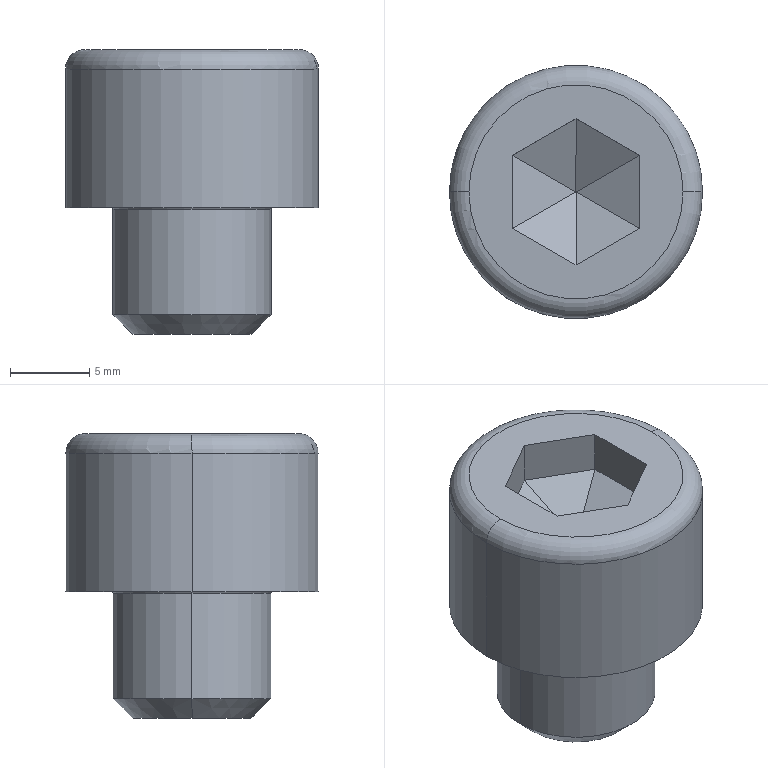Part | STEP file | Socket head cap screw M10x8 | 1 solid | 26 faces | box 16 x 16 x 18 mm | volume 2409 mm3 | plane 16 | torus 4 | cylinder 4 | cone 2 | commonest cylinder face diameters 10 x2 16 x2
STEP:
#1=CARTESIAN_POINT('',(-5.1,0.,0.));
#2=VERTEX_POINT('',#1);
#3=CARTESIAN_POINT('',(5.1,0.,0.));
#4=VERTEX_POINT('',#3);
#5=CARTESIAN_POINT('',(0.,0.,0.));
#6=DIRECTION('',(0.,0.,1.));
#7=DIRECTION('',(1.,0.,0.));
#8=AXIS2_PLACEMENT_3D('',#5,#6,#7);
#9=CIRCLE('',#8,5.1);
#10=EDGE_CURVE('',#2,#4,#9,.T.);
#11=ORIENTED_EDGE('',*,*,#10,.F.);
#12=CARTESIAN_POINT('',(-5.,0.,-0.1));
#13=VERTEX_POINT('',#12);
#14=CARTESIAN_POINT('',(-5.1,0.,-0.1));
#15=DIRECTION('',(0.,1.,0.));
#16=DIRECTION('',(-1.,0.,0.));
#17=AXIS2_PLACEMENT_3D('',#14,#15,#16);
#18=CIRCLE('',#17,0.1);
#19=EDGE_CURVE('',#2,#13,#18,.T.);
#20=ORIENTED_EDGE('',*,*,#19,.T.);
#21=CARTESIAN_POINT('',(5.,0.,-0.1));
#22=VERTEX_POINT('',#21);
#23=CARTESIAN_POINT('',(0.,0.,-0.1));
#24=DIRECTION('',(0.,0.,-1.));
#25=DIRECTION('',(1.,0.,0.));
#26=AXIS2_PLACEMENT_3D('',#23,#24,#25);
#27=CIRCLE('',#26,5.);
#28=EDGE_CURVE('',#22,#13,#27,.T.);
#29=ORIENTED_EDGE('',*,*,#28,.F.);
#30=CARTESIAN_POINT('',(5.1,0.,-0.1));
#31=DIRECTION('',(0.,-1.,0.));
#32=DIRECTION('',(0.,0.,-1.));
#33=AXIS2_PLACEMENT_3D('',#30,#31,#32);
#34=CIRCLE('',#33,0.1);
#35=EDGE_CURVE('',#4,#22,#34,.T.);
#36=ORIENTED_EDGE('',*,*,#35,.F.);
#37=EDGE_LOOP('',(#11,#20,#29,#36));
#38=FACE_OUTER_BOUND('',#37,.T.);
#39=CARTESIAN_POINT('',(0.,0.,-0.1));
#40=DIRECTION('',(0.,0.,1.));
#41=DIRECTION('',(1.,0.,0.));
#42=AXIS2_PLACEMENT_3D('',#39,#40,#41);
#43=TOROIDAL_SURFACE('',#42,5.1,0.1);
#44=ADVANCED_FACE('',(#38),#43,.F.);
#45=CARTESIAN_POINT('',(-8.,0.,8.769));
#46=VERTEX_POINT('',#45);
#47=CARTESIAN_POINT('',(8.,0.,8.769));
#48=VERTEX_POINT('',#47);
#49=CARTESIAN_POINT('',(0.,0.,8.769));
#50=DIRECTION('',(0.,0.,-1.));
#51=DIRECTION('',(1.,0.,0.));
#52=AXIS2_PLACEMENT_3D('',#49,#50,#51);
#53=CIRCLE('',#52,8.);
#54=EDGE_CURVE('',#46,#48,#53,.T.);
#55=ORIENTED_EDGE('',*,*,#54,.F.);
#56=CARTESIAN_POINT('',(-6.769,0.,10.));
#57=VERTEX_POINT('',#56);
#58=CARTESIAN_POINT('',(-6.769,0.,8.769));
#59=DIRECTION('',(0.,1.,0.));
#60=DIRECTION('',(-1.,0.,0.));
#61=AXIS2_PLACEMENT_3D('',#58,#59,#60);
#62=CIRCLE('',#61,1.231);
#63=EDGE_CURVE('',#46,#57,#62,.T.);
#64=ORIENTED_EDGE('',*,*,#63,.T.);
#65=CARTESIAN_POINT('',(6.769,0.,10.));
#66=VERTEX_POINT('',#65);
#67=CARTESIAN_POINT('',(0.,0.,10.));
#68=DIRECTION('',(0.,0.,1.));
#69=DIRECTION('',(1.,0.,0.));
#70=AXIS2_PLACEMENT_3D('',#67,#68,#69);
#71=CIRCLE('',#70,6.769);
#72=EDGE_CURVE('',#66,#57,#71,.T.);
#73=ORIENTED_EDGE('',*,*,#72,.F.);
#74=CARTESIAN_POINT('',(6.769,0.,8.769));
#75=DIRECTION('',(0.,-1.,0.));
#76=DIRECTION('',(0.,0.,-1.));
#77=AXIS2_PLACEMENT_3D('',#74,#75,#76);
#78=CIRCLE('',#77,1.231);
#79=EDGE_CURVE('',#48,#66,#78,.T.);
#80=ORIENTED_EDGE('',*,*,#79,.F.);
#81=EDGE_LOOP('',(#55,#64,#73,#80));
#82=FACE_OUTER_BOUND('',#81,.T.);
#83=CARTESIAN_POINT('',(0.,0.,8.769));
#84=DIRECTION('',(0.,0.,1.));
#85=DIRECTION('',(1.,0.,0.));
#86=AXIS2_PLACEMENT_3D('',#83,#84,#85);
#87=TOROIDAL_SURFACE('',#86,6.769,1.231);
#88=ADVANCED_FACE('',(#82),#87,.T.);
#89=CARTESIAN_POINT('',(-3.75,0.,-8.));
#90=VERTEX_POINT('',#89);
#91=CARTESIAN_POINT('',(3.75,0.,-8.));
#92=VERTEX_POINT('',#91);
#93=CARTESIAN_POINT('',(0.,0.,-8.));
#94=DIRECTION('',(0.,0.,-1.));
#95=DIRECTION('',(-1.,0.,0.));
#96=AXIS2_PLACEMENT_3D('',#93,#94,#95);
#97=CIRCLE('',#96,3.75);
#98=EDGE_CURVE('',#90,#92,#97,.T.);
#99=ORIENTED_EDGE('',*,*,#98,.F.);
#100=CARTESIAN_POINT('',(-5.,0.,-6.75));
#101=VERTEX_POINT('',#100);
#102=CARTESIAN_POINT('',(-3.75,0.,-8.));
#103=DIRECTION('',(-0.7071,0.,0.7071));
#104=VECTOR('',#103,1000.);
#105=LINE('',#102,#104);
#106=EDGE_CURVE('',#90,#101,#105,.T.);
#107=ORIENTED_EDGE('',*,*,#106,.T.);
#108=CARTESIAN_POINT('',(5.,0.,-6.75));
#109=VERTEX_POINT('',#108);
#110=CARTESIAN_POINT('',(0.,0.,-6.75));
#111=DIRECTION('',(0.,0.,1.));
#112=DIRECTION('',(-1.,0.,0.));
#113=AXIS2_PLACEMENT_3D('',#110,#111,#112);
#114=CIRCLE('',#113,5.);
#115=EDGE_CURVE('',#109,#101,#114,.T.);
#116=ORIENTED_EDGE('',*,*,#115,.F.);
#117=CARTESIAN_POINT('',(3.75,0.,-8.));
#118=DIRECTION('',(0.7071,0.,0.7071));
#119=VECTOR('',#118,1000.);
#120=LINE('',#117,#119);
#121=EDGE_CURVE('',#92,#109,#120,.T.);
#122=ORIENTED_EDGE('',*,*,#121,.F.);
#123=EDGE_LOOP('',(#99,#107,#116,#122));
#124=FACE_OUTER_BOUND('',#123,.T.);
#125=CARTESIAN_POINT('',(0.,0.,-8.));
#126=DIRECTION('',(0.,0.,1.));
#127=DIRECTION('',(1.,0.,0.));
#128=AXIS2_PLACEMENT_3D('',#125,#126,#127);
#129=CONICAL_SURFACE('',#128,3.75,0.7854);
#130=ADVANCED_FACE('',(#124),#129,.T.);
#131=ORIENTED_EDGE('',*,*,#115,.T.);
#132=CARTESIAN_POINT('',(-5.,0.,-8.));
#133=DIRECTION('',(0.,0.,1.));
#134=VECTOR('',#133,1000.);
#135=LINE('',#132,#134);
#136=EDGE_CURVE('',#101,#13,#135,.T.);
#137=ORIENTED_EDGE('',*,*,#136,.T.);
#138=CARTESIAN_POINT('',(0.,0.,-0.1));
#139=DIRECTION('',(0.,0.,-1.));
#140=DIRECTION('',(1.,0.,0.));
#141=AXIS2_PLACEMENT_3D('',#138,#139,#140);
#142=CIRCLE('',#141,5.);
#143=EDGE_CURVE('',#13,#22,#142,.T.);
#144=ORIENTED_EDGE('',*,*,#143,.T.);
#145=CARTESIAN_POINT('',(5.,0.,-8.));
#146=DIRECTION('',(0.,0.,1.));
#147=VECTOR('',#146,1000.);
#148=LINE('',#145,#147);
#149=EDGE_CURVE('',#109,#22,#148,.T.);
#150=ORIENTED_EDGE('',*,*,#149,.F.);
#151=EDGE_LOOP('',(#131,#137,#144,#150));
#152=FACE_OUTER_BOUND('',#151,.T.);
#153=CARTESIAN_POINT('',(0.,0.,-8.));
#154=DIRECTION('',(0.,0.,1.));
#155=DIRECTION('',(1.,0.,0.));
#156=AXIS2_PLACEMENT_3D('',#153,#154,#155);
#157=CYLINDRICAL_SURFACE('',#156,5.);
#158=ADVANCED_FACE('',(#152),#157,.T.);
#159=ORIENTED_EDGE('',*,*,#54,.T.);
#160=CARTESIAN_POINT('',(8.,0.,0.));
#161=VERTEX_POINT('',#160);
#162=CARTESIAN_POINT('',(8.,0.,10.));
#163=DIRECTION('',(0.,0.,-1.));
#164=VECTOR('',#163,1000.);
#165=LINE('',#162,#164);
#166=EDGE_CURVE('',#48,#161,#165,.T.);
#167=ORIENTED_EDGE('',*,*,#166,.T.);
#168=CARTESIAN_POINT('',(-8.,0.,0.));
#169=VERTEX_POINT('',#168);
#170=CARTESIAN_POINT('',(0.,0.,0.));
#171=DIRECTION('',(0.,0.,1.));
#172=DIRECTION('',(1.,0.,0.));
#173=AXIS2_PLACEMENT_3D('',#170,#171,#172);
#174=CIRCLE('',#173,8.);
#175=EDGE_CURVE('',#161,#169,#174,.T.);
#176=ORIENTED_EDGE('',*,*,#175,.T.);
#177=CARTESIAN_POINT('',(-8.,0.,10.));
#178=DIRECTION('',(0.,0.,-1.));
#179=VECTOR('',#178,1000.);
#180=LINE('',#177,#179);
#181=EDGE_CURVE('',#46,#169,#180,.T.);
#182=ORIENTED_EDGE('',*,*,#181,.F.);
#183=EDGE_LOOP('',(#159,#167,#176,#182));
#184=FACE_OUTER_BOUND('',#183,.T.);
#185=CARTESIAN_POINT('',(0.,0.,10.));
#186=DIRECTION('',(0.,0.,-1.));
#187=DIRECTION('',(-1.,0.,0.));
#188=AXIS2_PLACEMENT_3D('',#185,#186,#187);
#189=CYLINDRICAL_SURFACE('',#188,8.);
#190=ADVANCED_FACE('',(#184),#189,.T.);
#191=CARTESIAN_POINT('',(0.,0.,0.));
#192=DIRECTION('',(0.,0.,1.));
#193=DIRECTION('',(1.,0.,0.));
#194=AXIS2_PLACEMENT_3D('',#191,#192,#193);
#195=CIRCLE('',#194,5.1);
#196=EDGE_CURVE('',#4,#2,#195,.T.);
#197=ORIENTED_EDGE('',*,*,#196,.T.);
#198=ORIENTED_EDGE('',*,*,#10,.T.);
#199=EDGE_LOOP('',(#197,#198));
#200=FACE_BOUND('',#199,.T.);
#201=CARTESIAN_POINT('',(0.,0.,0.));
#202=DIRECTION('',(0.,0.,1.));
#203=DIRECTION('',(1.,0.,0.));
#204=AXIS2_PLACEMENT_3D('',#201,#202,#203);
#205=CIRCLE('',#204,8.);
#206=EDGE_CURVE('',#169,#161,#205,.T.);
#207=ORIENTED_EDGE('',*,*,#206,.F.);
#208=ORIENTED_EDGE('',*,*,#175,.F.);
#209=EDGE_LOOP('',(#207,#208));
#210=FACE_OUTER_BOUND('',#209,.T.);
#211=CARTESIAN_POINT('',(0.,0.,0.));
#212=DIRECTION('',(0.,0.,1.));
#213=DIRECTION('',(1.,0.,0.));
#214=AXIS2_PLACEMENT_3D('',#211,#212,#213);
#215=PLANE('',#214);
#216=ADVANCED_FACE('',(#200,#210),#215,.F.);
#217=ORIENTED_EDGE('',*,*,#166,.F.);
#218=CARTESIAN_POINT('',(0.,0.,8.769));
#219=DIRECTION('',(0.,0.,-1.));
#220=DIRECTION('',(1.,0.,0.));
#221=AXIS2_PLACEMENT_3D('',#218,#219,#220);
#222=CIRCLE('',#221,8.);
#223=EDGE_CURVE('',#48,#46,#222,.T.);
#224=ORIENTED_EDGE('',*,*,#223,.T.);
#225=ORIENTED_EDGE('',*,*,#181,.T.);
#226=ORIENTED_EDGE('',*,*,#206,.T.);
#227=EDGE_LOOP('',(#217,#224,#225,#226));
#228=FACE_OUTER_BOUND('',#227,.T.);
#229=CARTESIAN_POINT('',(0.,0.,10.));
#230=DIRECTION('',(0.,0.,-1.));
#231=DIRECTION('',(-1.,0.,0.));
#232=AXIS2_PLACEMENT_3D('',#229,#230,#231);
#233=CYLINDRICAL_SURFACE('',#232,8.);
#234=ADVANCED_FACE('',(#228),#233,.T.);
#235=ORIENTED_EDGE('',*,*,#72,.T.);
#236=CARTESIAN_POINT('',(0.,0.,10.));
#237=DIRECTION('',(0.,0.,1.));
#238=DIRECTION('',(1.,0.,0.));
#239=AXIS2_PLACEMENT_3D('',#236,#237,#238);
#240=CIRCLE('',#239,6.769);
#241=EDGE_CURVE('',#57,#66,#240,.T.);
#242=ORIENTED_EDGE('',*,*,#241,.T.);
#243=EDGE_LOOP('',(#235,#242));
#244=FACE_OUTER_BOUND('',#243,.T.);
#245=CARTESIAN_POINT('',(4.,-2.309,10.));
#246=VERTEX_POINT('',#245);
#247=CARTESIAN_POINT('',(4.,2.309,10.));
#248=VERTEX_POINT('',#247);
#249=CARTESIAN_POINT('',(4.,-2.309,10.));
#250=DIRECTION('',(0.,1.,0.));
#251=VECTOR('',#250,1000.);
#252=LINE('',#249,#251);
#253=EDGE_CURVE('',#246,#248,#252,.T.);
#254=ORIENTED_EDGE('',*,*,#253,.F.);
#255=CARTESIAN_POINT('',(0.,-4.619,10.));
#256=VERTEX_POINT('',#255);
#257=CARTESIAN_POINT('',(0.,-4.619,10.));
#258=DIRECTION('',(0.866,0.5,0.));
#259=VECTOR('',#258,1000.);
#260=LINE('',#257,#259);
#261=EDGE_CURVE('',#256,#246,#260,.T.);
#262=ORIENTED_EDGE('',*,*,#261,.F.);
#263=CARTESIAN_POINT('',(-4.,-2.309,10.));
#264=VERTEX_POINT('',#263);
#265=CARTESIAN_POINT('',(-4.,-2.309,10.));
#266=DIRECTION('',(0.866,-0.5,0.));
#267=VECTOR('',#266,1000.);
#268=LINE('',#265,#267);
#269=EDGE_CURVE('',#264,#256,#268,.T.);
#270=ORIENTED_EDGE('',*,*,#269,.F.);
#271=CARTESIAN_POINT('',(-4.,2.309,10.));
#272=VERTEX_POINT('',#271);
#273=CARTESIAN_POINT('',(-4.,2.309,10.));
#274=DIRECTION('',(0.,-1.,0.));
#275=VECTOR('',#274,1000.);
#276=LINE('',#273,#275);
#277=EDGE_CURVE('',#272,#264,#276,.T.);
#278=ORIENTED_EDGE('',*,*,#277,.F.);
#279=CARTESIAN_POINT('',(0.,4.619,10.));
#280=VERTEX_POINT('',#279);
#281=CARTESIAN_POINT('',(0.,4.619,10.));
#282=DIRECTION('',(-0.866,-0.5,0.));
#283=VECTOR('',#282,1000.);
#284=LINE('',#281,#283);
#285=EDGE_CURVE('',#280,#272,#284,.T.);
#286=ORIENTED_EDGE('',*,*,#285,.F.);
#287=CARTESIAN_POINT('',(4.,2.309,10.));
#288=DIRECTION('',(-0.866,0.5,0.));
#289=VECTOR('',#288,1000.);
#290=LINE('',#287,#289);
#291=EDGE_CURVE('',#248,#280,#290,.T.);
#292=ORIENTED_EDGE('',*,*,#291,.F.);
#293=EDGE_LOOP('',(#254,#262,#270,#278,#286,#292));
#294=FACE_BOUND('',#293,.T.);
#295=CARTESIAN_POINT('',(0.,0.,10.));
#296=DIRECTION('',(0.,0.,1.));
#297=DIRECTION('',(1.,0.,0.));
#298=AXIS2_PLACEMENT_3D('',#295,#296,#297);
#299=PLANE('',#298);
#300=ADVANCED_FACE('',(#244,#294),#299,.T.);
#301=CARTESIAN_POINT('',(4.,2.309,7.305));
#302=VERTEX_POINT('',#301);
#303=CARTESIAN_POINT('',(4.,2.309,5.));
#304=DIRECTION('',(0.,0.,1.));
#305=VECTOR('',#304,1000.);
#306=LINE('',#303,#305);
#307=EDGE_CURVE('',#302,#248,#306,.T.);
#308=ORIENTED_EDGE('',*,*,#307,.F.);
#309=CARTESIAN_POINT('',(4.,-2.309,7.305));
#310=VERTEX_POINT('',#309);
#311=CARTESIAN_POINT('',(4.,-2.309,7.305));
#312=DIRECTION('',(0.,-1.,0.));
#313=VECTOR('',#312,1000.);
#314=LINE('',#311,#313);
#315=EDGE_CURVE('',#302,#310,#314,.T.);
#316=ORIENTED_EDGE('',*,*,#315,.T.);
#317=CARTESIAN_POINT('',(4.,-2.309,5.));
#318=DIRECTION('',(0.,0.,1.));
#319=VECTOR('',#318,1000.);
#320=LINE('',#317,#319);
#321=EDGE_CURVE('',#310,#246,#320,.T.);
#322=ORIENTED_EDGE('',*,*,#321,.T.);
#323=ORIENTED_EDGE('',*,*,#253,.T.);
#324=EDGE_LOOP('',(#308,#316,#322,#323));
#325=FACE_OUTER_BOUND('',#324,.T.);
#326=CARTESIAN_POINT('',(4.,-2.309,5.));
#327=DIRECTION('',(1.,0.,0.));
#328=DIRECTION('',(0.,1.,0.));
#329=AXIS2_PLACEMENT_3D('',#326,#327,#328);
#330=PLANE('',#329);
#331=ADVANCED_FACE('',(#325),#330,.F.);
#332=ORIENTED_EDGE('',*,*,#321,.F.);
#333=CARTESIAN_POINT('',(0.,-4.619,7.305));
#334=VERTEX_POINT('',#333);
#335=CARTESIAN_POINT('',(0.,-4.619,7.305));
#336=DIRECTION('',(-0.866,-0.5,0.));
#337=VECTOR('',#336,1000.);
#338=LINE('',#335,#337);
#339=EDGE_CURVE('',#310,#334,#338,.T.);
#340=ORIENTED_EDGE('',*,*,#339,.T.);
#341=CARTESIAN_POINT('',(0.,-4.619,5.));
#342=DIRECTION('',(0.,0.,1.));
#343=VECTOR('',#342,1000.);
#344=LINE('',#341,#343);
#345=EDGE_CURVE('',#334,#256,#344,.T.);
#346=ORIENTED_EDGE('',*,*,#345,.T.);
#347=ORIENTED_EDGE('',*,*,#261,.T.);
#348=EDGE_LOOP('',(#332,#340,#346,#347));
#349=FACE_OUTER_BOUND('',#348,.T.);
#350=CARTESIAN_POINT('',(0.,-4.619,5.));
#351=DIRECTION('',(0.5,-0.866,0.));
#352=DIRECTION('',(0.866,0.5,0.));
#353=AXIS2_PLACEMENT_3D('',#350,#351,#352);
#354=PLANE('',#353);
#355=ADVANCED_FACE('',(#349),#354,.F.);
#356=ORIENTED_EDGE('',*,*,#345,.F.);
#357=CARTESIAN_POINT('',(-4.,-2.309,7.305));
#358=VERTEX_POINT('',#357);
#359=CARTESIAN_POINT('',(-4.,-2.309,7.305));
#360=DIRECTION('',(-0.866,0.5,0.));
#361=VECTOR('',#360,1000.);
#362=LINE('',#359,#361);
#363=EDGE_CURVE('',#334,#358,#362,.T.);
#364=ORIENTED_EDGE('',*,*,#363,.T.);
#365=CARTESIAN_POINT('',(-4.,-2.309,5.));
#366=DIRECTION('',(0.,0.,1.));
#367=VECTOR('',#366,1000.);
#368=LINE('',#365,#367);
#369=EDGE_CURVE('',#358,#264,#368,.T.);
#370=ORIENTED_EDGE('',*,*,#369,.T.);
#371=ORIENTED_EDGE('',*,*,#269,.T.);
#372=EDGE_LOOP('',(#356,#364,#370,#371));
#373=FACE_OUTER_BOUND('',#372,.T.);
#374=CARTESIAN_POINT('',(-4.,-2.309,5.));
#375=DIRECTION('',(-0.5,-0.866,0.));
#376=DIRECTION('',(0.866,-0.5,0.));
#377=AXIS2_PLACEMENT_3D('',#374,#375,#376);
#378=PLANE('',#377);
#379=ADVANCED_FACE('',(#373),#378,.F.);
#380=ORIENTED_EDGE('',*,*,#369,.F.);
#381=CARTESIAN_POINT('',(-4.,2.309,7.305));
#382=VERTEX_POINT('',#381);
#383=CARTESIAN_POINT('',(-4.,2.309,7.305));
#384=DIRECTION('',(0.,1.,0.));
#385=VECTOR('',#384,1000.);
#386=LINE('',#383,#385);
#387=EDGE_CURVE('',#358,#382,#386,.T.);
#388=ORIENTED_EDGE('',*,*,#387,.T.);
#389=CARTESIAN_POINT('',(-4.,2.309,5.));
#390=DIRECTION('',(0.,0.,1.));
#391=VECTOR('',#390,1000.);
#392=LINE('',#389,#391);
#393=EDGE_CURVE('',#382,#272,#392,.T.);
#394=ORIENTED_EDGE('',*,*,#393,.T.);
#395=ORIENTED_EDGE('',*,*,#277,.T.);
#396=EDGE_LOOP('',(#380,#388,#394,#395));
#397=FACE_OUTER_BOUND('',#396,.T.);
#398=CARTESIAN_POINT('',(-4.,2.309,5.));
#399=DIRECTION('',(-1.,0.,0.));
#400=DIRECTION('',(0.,0.,1.));
#401=AXIS2_PLACEMENT_3D('',#398,#399,#400);
#402=PLANE('',#401);
#403=ADVANCED_FACE('',(#397),#402,.F.);
#404=ORIENTED_EDGE('',*,*,#393,.F.);
#405=CARTESIAN_POINT('',(0.,4.619,7.305));
#406=VERTEX_POINT('',#405);
#407=CARTESIAN_POINT('',(0.,4.619,7.305));
#408=DIRECTION('',(0.866,0.5,0.));
#409=VECTOR('',#408,1000.);
#410=LINE('',#407,#409);
#411=EDGE_CURVE('',#382,#406,#410,.T.);
#412=ORIENTED_EDGE('',*,*,#411,.T.);
#413=CARTESIAN_POINT('',(0.,4.619,5.));
#414=DIRECTION('',(0.,0.,1.));
#415=VECTOR('',#414,1000.);
#416=LINE('',#413,#415);
#417=EDGE_CURVE('',#406,#280,#416,.T.);
#418=ORIENTED_EDGE('',*,*,#417,.T.);
#419=ORIENTED_EDGE('',*,*,#285,.T.);
#420=EDGE_LOOP('',(#404,#412,#418,#419));
#421=FACE_OUTER_BOUND('',#420,.T.);
#422=CARTESIAN_POINT('',(0.,4.619,5.));
#423=DIRECTION('',(-0.5,0.866,0.));
#424=DIRECTION('',(-0.866,-0.5,0.));
#425=AXIS2_PLACEMENT_3D('',#422,#423,#424);
#426=PLANE('',#425);
#427=ADVANCED_FACE('',(#421),#426,.F.);
#428=ORIENTED_EDGE('',*,*,#417,.F.);
#429=CARTESIAN_POINT('',(4.,2.309,7.305));
#430=DIRECTION('',(0.866,-0.5,0.));
#431=VECTOR('',#430,1000.);
#432=LINE('',#429,#431);
#433=EDGE_CURVE('',#406,#302,#432,.T.);
#434=ORIENTED_EDGE('',*,*,#433,.T.);
#435=ORIENTED_EDGE('',*,*,#307,.T.);
#436=ORIENTED_EDGE('',*,*,#291,.T.);
#437=EDGE_LOOP('',(#428,#434,#435,#436));
#438=FACE_OUTER_BOUND('',#437,.T.);
#439=CARTESIAN_POINT('',(4.,2.309,5.));
#440=DIRECTION('',(0.5,0.866,0.));
#441=DIRECTION('',(-0.866,0.5,0.));
#442=AXIS2_PLACEMENT_3D('',#439,#440,#441);
#443=PLANE('',#442);
#444=ADVANCED_FACE('',(#438),#443,.F.);
#445=CARTESIAN_POINT('',(0.,0.007851,5.));
#446=VERTEX_POINT('',#445);
#447=CARTESIAN_POINT('',(-0.006799,0.003926,5.));
#448=VERTEX_POINT('',#447);
#449=CARTESIAN_POINT('',(-0.0034,0.005888,5.));
#450=DIRECTION('',(-0.866,-0.5,0.));
#451=VECTOR('',#450,1000.);
#452=LINE('',#449,#451);
#453=EDGE_CURVE('',#446,#448,#452,.T.);
#454=ORIENTED_EDGE('',*,*,#453,.T.);
#455=CARTESIAN_POINT('',(-0.006799,-0.003926,5.));
#456=VERTEX_POINT('',#455);
#457=CARTESIAN_POINT('',(-0.006799,0.,5.));
#458=DIRECTION('',(0.,-1.,0.));
#459=VECTOR('',#458,1000.);
#460=LINE('',#457,#459);
#461=EDGE_CURVE('',#448,#456,#460,.T.);
#462=ORIENTED_EDGE('',*,*,#461,.T.);
#463=CARTESIAN_POINT('',(0.,-0.007851,5.));
#464=VERTEX_POINT('',#463);
#465=CARTESIAN_POINT('',(-0.0034,-0.005888,5.));
#466=DIRECTION('',(0.866,-0.5,0.));
#467=VECTOR('',#466,1000.);
#468=LINE('',#465,#467);
#469=EDGE_CURVE('',#456,#464,#468,.T.);
#470=ORIENTED_EDGE('',*,*,#469,.T.);
#471=CARTESIAN_POINT('',(0.006799,-0.003926,5.));
#472=VERTEX_POINT('',#471);
#473=CARTESIAN_POINT('',(0.0034,-0.005888,5.));
#474=DIRECTION('',(0.866,0.5,0.));
#475=VECTOR('',#474,1000.);
#476=LINE('',#473,#475);
#477=EDGE_CURVE('',#464,#472,#476,.T.);
#478=ORIENTED_EDGE('',*,*,#477,.T.);
#479=CARTESIAN_POINT('',(0.006799,0.003926,5.));
#480=VERTEX_POINT('',#479);
#481=CARTESIAN_POINT('',(0.006799,0.,5.));
#482=DIRECTION('',(0.,1.,0.));
#483=VECTOR('',#482,1000.);
#484=LINE('',#481,#483);
#485=EDGE_CURVE('',#472,#480,#484,.T.);
#486=ORIENTED_EDGE('',*,*,#485,.T.);
#487=CARTESIAN_POINT('',(0.0034,0.005888,5.));
#488=DIRECTION('',(-0.866,0.5,0.));
#489=VECTOR('',#488,1000.);
#490=LINE('',#487,#489);
#491=EDGE_CURVE('',#480,#446,#490,.T.);
#492=ORIENTED_EDGE('',*,*,#491,.T.);
#493=EDGE_LOOP('',(#454,#462,#470,#478,#486,#492));
#494=FACE_OUTER_BOUND('',#493,.T.);
#495=CARTESIAN_POINT('',(0.,0.,5.));
#496=DIRECTION('',(0.,0.,1.));
#497=DIRECTION('',(1.,0.,0.));
#498=AXIS2_PLACEMENT_3D('',#495,#496,#497);
#499=PLANE('',#498);
#500=ADVANCED_FACE('',(#494),#499,.T.);
#501=ORIENTED_EDGE('',*,*,#136,.F.);
#502=CARTESIAN_POINT('',(0.,0.,-6.75));
#503=DIRECTION('',(0.,0.,1.));
#504=DIRECTION('',(-1.,0.,0.));
#505=AXIS2_PLACEMENT_3D('',#502,#503,#504);
#506=CIRCLE('',#505,5.);
#507=EDGE_CURVE('',#101,#109,#506,.T.);
#508=ORIENTED_EDGE('',*,*,#507,.T.);
#509=ORIENTED_EDGE('',*,*,#149,.T.);
#510=ORIENTED_EDGE('',*,*,#28,.T.);
#511=EDGE_LOOP('',(#501,#508,#509,#510));
#512=FACE_OUTER_BOUND('',#511,.T.);
#513=CARTESIAN_POINT('',(0.,0.,-8.));
#514=DIRECTION('',(0.,0.,1.));
#515=DIRECTION('',(1.,0.,0.));
#516=AXIS2_PLACEMENT_3D('',#513,#514,#515);
#517=CYLINDRICAL_SURFACE('',#516,5.);
#518=ADVANCED_FACE('',(#512),#517,.T.);
#519=CARTESIAN_POINT('',(0.,0.,-8.));
#520=DIRECTION('',(0.,0.,-1.));
#521=DIRECTION('',(-1.,0.,0.));
#522=AXIS2_PLACEMENT_3D('',#519,#520,#521);
#523=CIRCLE('',#522,3.75);
#524=EDGE_CURVE('',#92,#90,#523,.T.);
#525=ORIENTED_EDGE('',*,*,#524,.T.);
#526=ORIENTED_EDGE('',*,*,#98,.T.);
#527=EDGE_LOOP('',(#525,#526));
#528=FACE_OUTER_BOUND('',#527,.T.);
#529=CARTESIAN_POINT('',(0.,0.,-8.));
#530=DIRECTION('',(0.,0.,-1.));
#531=DIRECTION('',(-1.,0.,0.));
#532=AXIS2_PLACEMENT_3D('',#529,#530,#531);
#533=PLANE('',#532);
#534=ADVANCED_FACE('',(#528),#533,.T.);
#535=ORIENTED_EDGE('',*,*,#106,.F.);
#536=ORIENTED_EDGE('',*,*,#524,.F.);
#537=ORIENTED_EDGE('',*,*,#121,.T.);
#538=ORIENTED_EDGE('',*,*,#507,.F.);
#539=EDGE_LOOP('',(#535,#536,#537,#538));
#540=FACE_OUTER_BOUND('',#539,.T.);
#541=CARTESIAN_POINT('',(0.,0.,-8.));
#542=DIRECTION('',(0.,0.,1.));
#543=DIRECTION('',(1.,0.,0.));
#544=AXIS2_PLACEMENT_3D('',#541,#542,#543);
#545=CONICAL_SURFACE('',#544,3.75,0.7854);
#546=ADVANCED_FACE('',(#540),#545,.T.);
#547=ORIENTED_EDGE('',*,*,#63,.F.);
#548=ORIENTED_EDGE('',*,*,#223,.F.);
#549=ORIENTED_EDGE('',*,*,#79,.T.);
#550=ORIENTED_EDGE('',*,*,#241,.F.);
#551=EDGE_LOOP('',(#547,#548,#549,#550));
#552=FACE_OUTER_BOUND('',#551,.T.);
#553=CARTESIAN_POINT('',(0.,0.,8.769));
#554=DIRECTION('',(0.,0.,1.));
#555=DIRECTION('',(1.,0.,0.));
#556=AXIS2_PLACEMENT_3D('',#553,#554,#555);
#557=TOROIDAL_SURFACE('',#556,6.769,1.231);
#558=ADVANCED_FACE('',(#552),#557,.T.);
#559=CARTESIAN_POINT('',(0.005439,-0.00314,4.999));
#560=DIRECTION('',(-0.7746,0.4472,-0.4472));
#561=VECTOR('',#560,1000.);
#562=LINE('',#559,#561);
#563=EDGE_CURVE('',#310,#472,#562,.T.);
#564=ORIENTED_EDGE('',*,*,#563,.F.);
#565=ORIENTED_EDGE('',*,*,#315,.F.);
#566=CARTESIAN_POINT('',(0.005439,0.00314,4.999));
#567=DIRECTION('',(0.7746,0.4472,0.4472));
#568=VECTOR('',#567,1000.);
#569=LINE('',#566,#568);
#570=EDGE_CURVE('',#480,#302,#569,.T.);
#571=ORIENTED_EDGE('',*,*,#570,.F.);
#572=ORIENTED_EDGE('',*,*,#485,.F.);
#573=EDGE_LOOP('',(#564,#565,#571,#572));
#574=FACE_OUTER_BOUND('',#573,.T.);
#575=CARTESIAN_POINT('',(0.006799,0.,5.));
#576=DIRECTION('',(0.5,0.,-0.866));
#577=DIRECTION('',(0.,1.,0.));
#578=AXIS2_PLACEMENT_3D('',#575,#576,#577);
#579=PLANE('',#578);
#580=ADVANCED_FACE('',(#574),#579,.F.);
#581=ORIENTED_EDGE('',*,*,#570,.T.);
#582=ORIENTED_EDGE('',*,*,#433,.F.);
#583=CARTESIAN_POINT('',(0.,0.006281,4.999));
#584=DIRECTION('',(0.,0.8944,0.4472));
#585=VECTOR('',#584,1000.);
#586=LINE('',#583,#585);
#587=EDGE_CURVE('',#446,#406,#586,.T.);
#588=ORIENTED_EDGE('',*,*,#587,.F.);
#589=ORIENTED_EDGE('',*,*,#491,.F.);
#590=EDGE_LOOP('',(#581,#582,#588,#589));
#591=FACE_OUTER_BOUND('',#590,.T.);
#592=CARTESIAN_POINT('',(0.0034,0.005888,5.));
#593=DIRECTION('',(0.25,0.433,-0.866));
#594=DIRECTION('',(-0.866,0.5,0.));
#595=AXIS2_PLACEMENT_3D('',#592,#593,#594);
#596=PLANE('',#595);
#597=ADVANCED_FACE('',(#591),#596,.F.);
#598=ORIENTED_EDGE('',*,*,#563,.T.);
#599=ORIENTED_EDGE('',*,*,#477,.F.);
#600=CARTESIAN_POINT('',(0.,-0.006281,4.999));
#601=DIRECTION('',(0.,0.8944,-0.4472));
#602=VECTOR('',#601,1000.);
#603=LINE('',#600,#602);
#604=EDGE_CURVE('',#334,#464,#603,.T.);
#605=ORIENTED_EDGE('',*,*,#604,.F.);
#606=ORIENTED_EDGE('',*,*,#339,.F.);
#607=EDGE_LOOP('',(#598,#599,#605,#606));
#608=FACE_OUTER_BOUND('',#607,.T.);
#609=CARTESIAN_POINT('',(0.0034,-0.005888,5.));
#610=DIRECTION('',(0.25,-0.433,-0.866));
#611=DIRECTION('',(0.866,0.5,0.));
#612=AXIS2_PLACEMENT_3D('',#609,#610,#611);
#613=PLANE('',#612);
#614=ADVANCED_FACE('',(#608),#613,.F.);
#615=ORIENTED_EDGE('',*,*,#587,.T.);
#616=ORIENTED_EDGE('',*,*,#411,.F.);
#617=CARTESIAN_POINT('',(-0.005439,0.00314,4.999));
#618=DIRECTION('',(-0.7746,0.4472,0.4472));
#619=VECTOR('',#618,1000.);
#620=LINE('',#617,#619);
#621=EDGE_CURVE('',#448,#382,#620,.T.);
#622=ORIENTED_EDGE('',*,*,#621,.F.);
#623=ORIENTED_EDGE('',*,*,#453,.F.);
#624=EDGE_LOOP('',(#615,#616,#622,#623));
#625=FACE_OUTER_BOUND('',#624,.T.);
#626=CARTESIAN_POINT('',(-0.0034,0.005888,5.));
#627=DIRECTION('',(-0.25,0.433,-0.866));
#628=DIRECTION('',(-0.866,-0.5,0.));
#629=AXIS2_PLACEMENT_3D('',#626,#627,#628);
#630=PLANE('',#629);
#631=ADVANCED_FACE('',(#625),#630,.F.);
#632=ORIENTED_EDGE('',*,*,#604,.T.);
#633=ORIENTED_EDGE('',*,*,#469,.F.);
#634=CARTESIAN_POINT('',(-0.005439,-0.00314,4.999));
#635=DIRECTION('',(0.7746,0.4472,-0.4472));
#636=VECTOR('',#635,1000.);
#637=LINE('',#634,#636);
#638=EDGE_CURVE('',#358,#456,#637,.T.);
#639=ORIENTED_EDGE('',*,*,#638,.F.);
#640=ORIENTED_EDGE('',*,*,#363,.F.);
#641=EDGE_LOOP('',(#632,#633,#639,#640));
#642=FACE_OUTER_BOUND('',#641,.T.);
#643=CARTESIAN_POINT('',(-0.0034,-0.005888,5.));
#644=DIRECTION('',(-0.25,-0.433,-0.866));
#645=DIRECTION('',(0.866,-0.5,0.));
#646=AXIS2_PLACEMENT_3D('',#643,#644,#645);
#647=PLANE('',#646);
#648=ADVANCED_FACE('',(#642),#647,.F.);
#649=ORIENTED_EDGE('',*,*,#621,.T.);
#650=ORIENTED_EDGE('',*,*,#387,.F.);
#651=ORIENTED_EDGE('',*,*,#638,.T.);
#652=ORIENTED_EDGE('',*,*,#461,.F.);
#653=EDGE_LOOP('',(#649,#650,#651,#652));
#654=FACE_OUTER_BOUND('',#653,.T.);
#655=CARTESIAN_POINT('',(-0.006799,0.,5.));
#656=DIRECTION('',(-0.5,0.,-0.866));
#657=DIRECTION('',(0.,-1.,0.));
#658=AXIS2_PLACEMENT_3D('',#655,#656,#657);
#659=PLANE('',#658);
#660=ADVANCED_FACE('',(#654),#659,.F.);
#661=ORIENTED_EDGE('',*,*,#19,.F.);
#662=ORIENTED_EDGE('',*,*,#196,.F.);
#663=ORIENTED_EDGE('',*,*,#35,.T.);
#664=ORIENTED_EDGE('',*,*,#143,.F.);
#665=EDGE_LOOP('',(#661,#662,#663,#664));
#666=FACE_OUTER_BOUND('',#665,.T.);
#667=CARTESIAN_POINT('',(0.,0.,-0.1));
#668=DIRECTION('',(0.,0.,1.));
#669=DIRECTION('',(1.,0.,0.));
#670=AXIS2_PLACEMENT_3D('',#667,#668,#669);
#671=TOROIDAL_SURFACE('',#670,5.1,0.1);
#672=ADVANCED_FACE('',(#666),#671,.F.);
#673=CLOSED_SHELL('',(#44,#88,#130,#158,#190,#216,#234,#300,#331,#355,#379,#403,#427,#444,#500,#518,#534,#546,#558,#580,#597,#614,#631,#648,#660,#672));
#674=MANIFOLD_SOLID_BREP('',#673);
#675=CARTESIAN_POINT('',(0.,0.,0.));
#676=DIRECTION('',(0.,0.,1.));
#677=DIRECTION('',(1.,0.,0.));
#678=AXIS2_PLACEMENT_3D('',#675,#676,#677);
#679=(LENGTH_UNIT()NAMED_UNIT(*)SI_UNIT(.MILLI.,.METRE.));
#680=UNCERTAINTY_MEASURE_WITH_UNIT(LENGTH_MEASURE(0.00001),#679,'','');
#681=(NAMED_UNIT(*)PLANE_ANGLE_UNIT()SI_UNIT($,.RADIAN.));
#682=(NAMED_UNIT(*)SI_UNIT($,.STERADIAN.)SOLID_ANGLE_UNIT());
#683=(GEOMETRIC_REPRESENTATION_CONTEXT(3)GLOBAL_UNCERTAINTY_ASSIGNED_CONTEXT((#680))GLOBAL_UNIT_ASSIGNED_CONTEXT((#679,#681,#682))REPRESENTATION_CONTEXT('',''));
#684=ADVANCED_BREP_SHAPE_REPRESENTATION('',(#674,#678),#683);